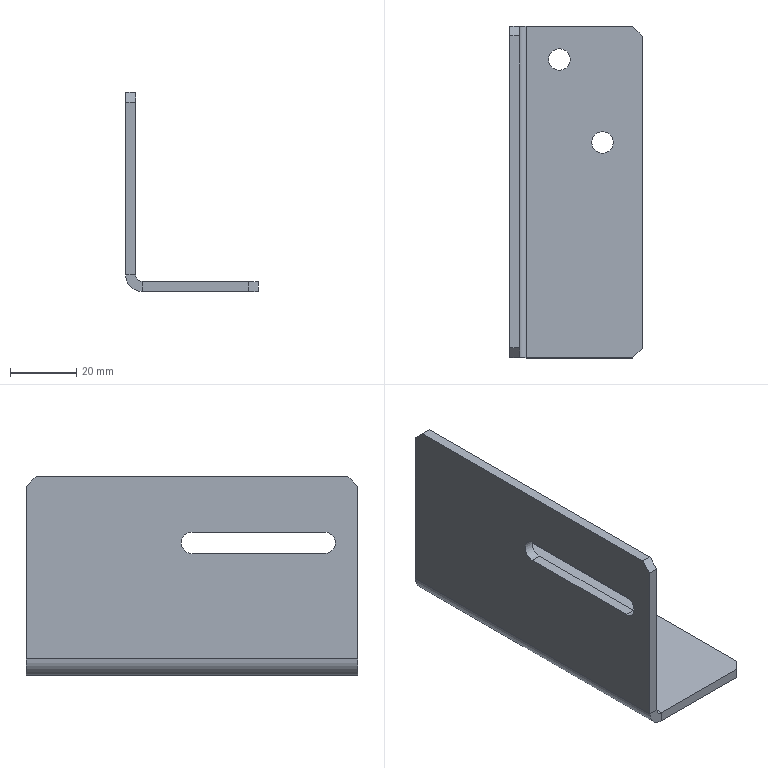Part | SolidWorks | features Chamfer 1, EdgeFlange 1, FlatPattern 1, ICE 1, SMBaseFlange 1, SheetMetal 1 | 1 solid | 26 faces | box 40 x 100 x 60 mm | volume 27517 mm3 | plane 18 | cylinder 8 | commonest cylinder face diameters 6.5 x6 4 x1 10 x1
STEP:
#1=CARTESIAN_POINT('',(-8.25,40.,-3.));
#2=VERTEX_POINT('',#1);
#3=CARTESIAN_POINT('',(-1.75,40.,-3.));
#4=VERTEX_POINT('',#3);
#5=CARTESIAN_POINT('',(-5.,40.,-3.));
#6=DIRECTION('',(0.,0.,1.));
#7=DIRECTION('',(1.,0.,0.));
#8=AXIS2_PLACEMENT_3D('',#5,#6,#7);
#9=CIRCLE('',#8,3.25);
#10=EDGE_CURVE('',#2,#4,#9,.T.);
#11=ORIENTED_EDGE('',*,*,#10,.F.);
#12=CARTESIAN_POINT('',(-8.25,40.,0.));
#13=VERTEX_POINT('',#12);
#14=CARTESIAN_POINT('',(-8.25,40.,-3.));
#15=DIRECTION('',(0.,0.,1.));
#16=VECTOR('',#15,1000.);
#17=LINE('',#14,#16);
#18=EDGE_CURVE('',#2,#13,#17,.T.);
#19=ORIENTED_EDGE('',*,*,#18,.T.);
#20=CARTESIAN_POINT('',(-1.75,40.,0.));
#21=VERTEX_POINT('',#20);
#22=CARTESIAN_POINT('',(-5.,40.,0.));
#23=DIRECTION('',(0.,0.,1.));
#24=DIRECTION('',(1.,0.,0.));
#25=AXIS2_PLACEMENT_3D('',#22,#23,#24);
#26=CIRCLE('',#25,3.25);
#27=EDGE_CURVE('',#13,#21,#26,.T.);
#28=ORIENTED_EDGE('',*,*,#27,.T.);
#29=CARTESIAN_POINT('',(-1.75,40.,-3.));
#30=DIRECTION('',(0.,0.,1.));
#31=VECTOR('',#30,1000.);
#32=LINE('',#29,#31);
#33=EDGE_CURVE('',#4,#21,#32,.T.);
#34=ORIENTED_EDGE('',*,*,#33,.F.);
#35=EDGE_LOOP('',(#11,#19,#28,#34));
#36=FACE_OUTER_BOUND('',#35,.T.);
#37=CARTESIAN_POINT('',(-5.,40.,-3.));
#38=DIRECTION('',(0.,0.,1.));
#39=DIRECTION('',(1.,0.,0.));
#40=AXIS2_PLACEMENT_3D('',#37,#38,#39);
#41=CYLINDRICAL_SURFACE('',#40,3.25);
#42=ADVANCED_FACE('',(#36),#41,.F.);
#43=CARTESIAN_POINT('',(4.75,15.,-3.));
#44=VERTEX_POINT('',#43);
#45=CARTESIAN_POINT('',(11.25,15.,-3.));
#46=VERTEX_POINT('',#45);
#47=CARTESIAN_POINT('',(8.,15.,-3.));
#48=DIRECTION('',(0.,0.,1.));
#49=DIRECTION('',(1.,0.,0.));
#50=AXIS2_PLACEMENT_3D('',#47,#48,#49);
#51=CIRCLE('',#50,3.25);
#52=EDGE_CURVE('',#44,#46,#51,.T.);
#53=ORIENTED_EDGE('',*,*,#52,.F.);
#54=CARTESIAN_POINT('',(4.75,15.,0.));
#55=VERTEX_POINT('',#54);
#56=CARTESIAN_POINT('',(4.75,15.,-3.));
#57=DIRECTION('',(0.,0.,1.));
#58=VECTOR('',#57,1000.);
#59=LINE('',#56,#58);
#60=EDGE_CURVE('',#44,#55,#59,.T.);
#61=ORIENTED_EDGE('',*,*,#60,.T.);
#62=CARTESIAN_POINT('',(11.25,15.,0.));
#63=VERTEX_POINT('',#62);
#64=CARTESIAN_POINT('',(8.,15.,0.));
#65=DIRECTION('',(0.,0.,1.));
#66=DIRECTION('',(1.,0.,0.));
#67=AXIS2_PLACEMENT_3D('',#64,#65,#66);
#68=CIRCLE('',#67,3.25);
#69=EDGE_CURVE('',#55,#63,#68,.T.);
#70=ORIENTED_EDGE('',*,*,#69,.T.);
#71=CARTESIAN_POINT('',(11.25,15.,-3.));
#72=DIRECTION('',(0.,0.,1.));
#73=VECTOR('',#72,1000.);
#74=LINE('',#71,#73);
#75=EDGE_CURVE('',#46,#63,#74,.T.);
#76=ORIENTED_EDGE('',*,*,#75,.F.);
#77=EDGE_LOOP('',(#53,#61,#70,#76));
#78=FACE_OUTER_BOUND('',#77,.T.);
#79=CARTESIAN_POINT('',(8.,15.,-3.));
#80=DIRECTION('',(0.,0.,1.));
#81=DIRECTION('',(1.,0.,0.));
#82=AXIS2_PLACEMENT_3D('',#79,#80,#81);
#83=CYLINDRICAL_SURFACE('',#82,3.25);
#84=ADVANCED_FACE('',(#78),#83,.F.);
#85=CARTESIAN_POINT('',(-15.,-50.,0.));
#86=VERTEX_POINT('',#85);
#87=CARTESIAN_POINT('',(17.,-50.,0.));
#88=VERTEX_POINT('',#87);
#89=CARTESIAN_POINT('',(17.,-50.,0.));
#90=DIRECTION('',(1.,0.,0.));
#91=VECTOR('',#90,1000.);
#92=LINE('',#89,#91);
#93=EDGE_CURVE('',#86,#88,#92,.T.);
#94=ORIENTED_EDGE('',*,*,#93,.F.);
#95=CARTESIAN_POINT('',(-15.,-50.,-3.));
#96=VERTEX_POINT('',#95);
#97=CARTESIAN_POINT('',(-15.,-50.,0.));
#98=DIRECTION('',(0.,0.,-1.));
#99=VECTOR('',#98,1000.);
#100=LINE('',#97,#99);
#101=EDGE_CURVE('',#86,#96,#100,.T.);
#102=ORIENTED_EDGE('',*,*,#101,.T.);
#103=CARTESIAN_POINT('',(17.,-50.,-3.));
#104=VERTEX_POINT('',#103);
#105=CARTESIAN_POINT('',(17.,-50.,-3.));
#106=DIRECTION('',(1.,0.,0.));
#107=VECTOR('',#106,1000.);
#108=LINE('',#105,#107);
#109=EDGE_CURVE('',#96,#104,#108,.T.);
#110=ORIENTED_EDGE('',*,*,#109,.T.);
#111=CARTESIAN_POINT('',(17.,-50.,-3.));
#112=DIRECTION('',(0.,0.,1.));
#113=VECTOR('',#112,1000.);
#114=LINE('',#111,#113);
#115=EDGE_CURVE('',#104,#88,#114,.T.);
#116=ORIENTED_EDGE('',*,*,#115,.T.);
#117=EDGE_LOOP('',(#94,#102,#110,#116));
#118=FACE_OUTER_BOUND('',#117,.T.);
#119=CARTESIAN_POINT('',(17.,-50.,-3.));
#120=DIRECTION('',(0.,-1.,0.));
#121=DIRECTION('',(0.,0.,-1.));
#122=AXIS2_PLACEMENT_3D('',#119,#120,#121);
#123=PLANE('',#122);
#124=ADVANCED_FACE('',(#118),#123,.T.);
#125=CARTESIAN_POINT('',(8.,15.,-3.));
#126=DIRECTION('',(0.,0.,1.));
#127=DIRECTION('',(1.,0.,0.));
#128=AXIS2_PLACEMENT_3D('',#125,#126,#127);
#129=CIRCLE('',#128,3.25);
#130=EDGE_CURVE('',#46,#44,#129,.T.);
#131=ORIENTED_EDGE('',*,*,#130,.T.);
#132=ORIENTED_EDGE('',*,*,#52,.T.);
#133=EDGE_LOOP('',(#131,#132));
#134=FACE_BOUND('',#133,.T.);
#135=CARTESIAN_POINT('',(-5.,40.,-3.));
#136=DIRECTION('',(0.,0.,1.));
#137=DIRECTION('',(1.,0.,0.));
#138=AXIS2_PLACEMENT_3D('',#135,#136,#137);
#139=CIRCLE('',#138,3.25);
#140=EDGE_CURVE('',#4,#2,#139,.T.);
#141=ORIENTED_EDGE('',*,*,#140,.T.);
#142=ORIENTED_EDGE('',*,*,#10,.T.);
#143=EDGE_LOOP('',(#141,#142));
#144=FACE_BOUND('',#143,.T.);
#145=CARTESIAN_POINT('',(-15.,50.,-3.));
#146=VERTEX_POINT('',#145);
#147=CARTESIAN_POINT('',(-15.,-50.,-3.));
#148=DIRECTION('',(0.,1.,0.));
#149=VECTOR('',#148,1000.);
#150=LINE('',#147,#149);
#151=EDGE_CURVE('',#96,#146,#150,.T.);
#152=ORIENTED_EDGE('',*,*,#151,.T.);
#153=CARTESIAN_POINT('',(17.,50.,-3.));
#154=VERTEX_POINT('',#153);
#155=CARTESIAN_POINT('',(17.,50.,-3.));
#156=DIRECTION('',(-1.,0.,0.));
#157=VECTOR('',#156,1000.);
#158=LINE('',#155,#157);
#159=EDGE_CURVE('',#154,#146,#158,.T.);
#160=ORIENTED_EDGE('',*,*,#159,.F.);
#161=CARTESIAN_POINT('',(20.,47.,-3.));
#162=VERTEX_POINT('',#161);
#163=CARTESIAN_POINT('',(20.,47.,-3.));
#164=DIRECTION('',(-0.7071,0.7071,0.));
#165=VECTOR('',#164,1000.);
#166=LINE('',#163,#165);
#167=EDGE_CURVE('',#162,#154,#166,.T.);
#168=ORIENTED_EDGE('',*,*,#167,.F.);
#169=CARTESIAN_POINT('',(20.,-47.,-3.));
#170=VERTEX_POINT('',#169);
#171=CARTESIAN_POINT('',(20.,-47.,-3.));
#172=DIRECTION('',(0.,1.,0.));
#173=VECTOR('',#172,1000.);
#174=LINE('',#171,#173);
#175=EDGE_CURVE('',#170,#162,#174,.T.);
#176=ORIENTED_EDGE('',*,*,#175,.F.);
#177=CARTESIAN_POINT('',(17.,-50.,-3.));
#178=DIRECTION('',(0.7071,0.7071,0.));
#179=VECTOR('',#178,1000.);
#180=LINE('',#177,#179);
#181=EDGE_CURVE('',#104,#170,#180,.T.);
#182=ORIENTED_EDGE('',*,*,#181,.F.);
#183=ORIENTED_EDGE('',*,*,#109,.F.);
#184=EDGE_LOOP('',(#152,#160,#168,#176,#182,#183));
#185=FACE_OUTER_BOUND('',#184,.T.);
#186=CARTESIAN_POINT('',(0.,0.,-3.));
#187=DIRECTION('',(0.,0.,1.));
#188=DIRECTION('',(1.,0.,0.));
#189=AXIS2_PLACEMENT_3D('',#186,#187,#188);
#190=PLANE('',#189);
#191=ADVANCED_FACE('',(#134,#144,#185),#190,.F.);
#192=CARTESIAN_POINT('',(-5.,40.,0.));
#193=DIRECTION('',(0.,0.,1.));
#194=DIRECTION('',(1.,0.,0.));
#195=AXIS2_PLACEMENT_3D('',#192,#193,#194);
#196=CIRCLE('',#195,3.25);
#197=EDGE_CURVE('',#21,#13,#196,.T.);
#198=ORIENTED_EDGE('',*,*,#197,.F.);
#199=ORIENTED_EDGE('',*,*,#27,.F.);
#200=EDGE_LOOP('',(#198,#199));
#201=FACE_BOUND('',#200,.T.);
#202=CARTESIAN_POINT('',(8.,15.,0.));
#203=DIRECTION('',(0.,0.,1.));
#204=DIRECTION('',(1.,0.,0.));
#205=AXIS2_PLACEMENT_3D('',#202,#203,#204);
#206=CIRCLE('',#205,3.25);
#207=EDGE_CURVE('',#63,#55,#206,.T.);
#208=ORIENTED_EDGE('',*,*,#207,.F.);
#209=ORIENTED_EDGE('',*,*,#69,.F.);
#210=EDGE_LOOP('',(#208,#209));
#211=FACE_BOUND('',#210,.T.);
#212=CARTESIAN_POINT('',(17.,50.,0.));
#213=VERTEX_POINT('',#212);
#214=CARTESIAN_POINT('',(-15.,50.,0.));
#215=VERTEX_POINT('',#214);
#216=CARTESIAN_POINT('',(17.,50.,0.));
#217=DIRECTION('',(-1.,0.,0.));
#218=VECTOR('',#217,1000.);
#219=LINE('',#216,#218);
#220=EDGE_CURVE('',#213,#215,#219,.T.);
#221=ORIENTED_EDGE('',*,*,#220,.T.);
#222=CARTESIAN_POINT('',(-15.,-50.,0.));
#223=DIRECTION('',(0.,1.,0.));
#224=VECTOR('',#223,1000.);
#225=LINE('',#222,#224);
#226=EDGE_CURVE('',#86,#215,#225,.T.);
#227=ORIENTED_EDGE('',*,*,#226,.F.);
#228=ORIENTED_EDGE('',*,*,#93,.T.);
#229=CARTESIAN_POINT('',(20.,-47.,0.));
#230=VERTEX_POINT('',#229);
#231=CARTESIAN_POINT('',(17.,-50.,0.));
#232=DIRECTION('',(0.7071,0.7071,0.));
#233=VECTOR('',#232,1000.);
#234=LINE('',#231,#233);
#235=EDGE_CURVE('',#88,#230,#234,.T.);
#236=ORIENTED_EDGE('',*,*,#235,.T.);
#237=CARTESIAN_POINT('',(20.,47.,0.));
#238=VERTEX_POINT('',#237);
#239=CARTESIAN_POINT('',(20.,-47.,0.));
#240=DIRECTION('',(0.,1.,0.));
#241=VECTOR('',#240,1000.);
#242=LINE('',#239,#241);
#243=EDGE_CURVE('',#230,#238,#242,.T.);
#244=ORIENTED_EDGE('',*,*,#243,.T.);
#245=CARTESIAN_POINT('',(20.,47.,0.));
#246=DIRECTION('',(-0.7071,0.7071,0.));
#247=VECTOR('',#246,1000.);
#248=LINE('',#245,#247);
#249=EDGE_CURVE('',#238,#213,#248,.T.);
#250=ORIENTED_EDGE('',*,*,#249,.T.);
#251=EDGE_LOOP('',(#221,#227,#228,#236,#244,#250));
#252=FACE_OUTER_BOUND('',#251,.T.);
#253=CARTESIAN_POINT('',(0.,0.,0.));
#254=DIRECTION('',(0.,0.,1.));
#255=DIRECTION('',(1.,0.,0.));
#256=AXIS2_PLACEMENT_3D('',#253,#254,#255);
#257=PLANE('',#256);
#258=ADVANCED_FACE('',(#201,#211,#252),#257,.T.);
#259=CARTESIAN_POINT('',(-15.,50.,0.));
#260=DIRECTION('',(0.,0.,-1.));
#261=VECTOR('',#260,1000.);
#262=LINE('',#259,#261);
#263=EDGE_CURVE('',#215,#146,#262,.T.);
#264=ORIENTED_EDGE('',*,*,#263,.F.);
#265=ORIENTED_EDGE('',*,*,#220,.F.);
#266=CARTESIAN_POINT('',(17.,50.,-3.));
#267=DIRECTION('',(0.,0.,1.));
#268=VECTOR('',#267,1000.);
#269=LINE('',#266,#268);
#270=EDGE_CURVE('',#154,#213,#269,.T.);
#271=ORIENTED_EDGE('',*,*,#270,.F.);
#272=ORIENTED_EDGE('',*,*,#159,.T.);
#273=EDGE_LOOP('',(#264,#265,#271,#272));
#274=FACE_OUTER_BOUND('',#273,.T.);
#275=CARTESIAN_POINT('',(17.,50.,-3.));
#276=DIRECTION('',(0.,1.,0.));
#277=DIRECTION('',(0.,0.,1.));
#278=AXIS2_PLACEMENT_3D('',#275,#276,#277);
#279=PLANE('',#278);
#280=ADVANCED_FACE('',(#274),#279,.T.);
#281=ORIENTED_EDGE('',*,*,#249,.F.);
#282=CARTESIAN_POINT('',(20.,47.,-3.));
#283=DIRECTION('',(0.,0.,1.));
#284=VECTOR('',#283,1000.);
#285=LINE('',#282,#284);
#286=EDGE_CURVE('',#162,#238,#285,.T.);
#287=ORIENTED_EDGE('',*,*,#286,.F.);
#288=ORIENTED_EDGE('',*,*,#167,.T.);
#289=ORIENTED_EDGE('',*,*,#270,.T.);
#290=EDGE_LOOP('',(#281,#287,#288,#289));
#291=FACE_OUTER_BOUND('',#290,.T.);
#292=CARTESIAN_POINT('',(20.,47.,-3.));
#293=DIRECTION('',(0.7071,0.7071,0.));
#294=DIRECTION('',(-0.7071,0.7071,0.));
#295=AXIS2_PLACEMENT_3D('',#292,#293,#294);
#296=PLANE('',#295);
#297=ADVANCED_FACE('',(#291),#296,.T.);
#298=ORIENTED_EDGE('',*,*,#243,.F.);
#299=CARTESIAN_POINT('',(20.,-47.,-3.));
#300=DIRECTION('',(0.,0.,1.));
#301=VECTOR('',#300,1000.);
#302=LINE('',#299,#301);
#303=EDGE_CURVE('',#170,#230,#302,.T.);
#304=ORIENTED_EDGE('',*,*,#303,.F.);
#305=ORIENTED_EDGE('',*,*,#175,.T.);
#306=ORIENTED_EDGE('',*,*,#286,.T.);
#307=EDGE_LOOP('',(#298,#304,#305,#306));
#308=FACE_OUTER_BOUND('',#307,.T.);
#309=CARTESIAN_POINT('',(20.,-47.,-3.));
#310=DIRECTION('',(1.,0.,0.));
#311=DIRECTION('',(0.,1.,0.));
#312=AXIS2_PLACEMENT_3D('',#309,#310,#311);
#313=PLANE('',#312);
#314=ADVANCED_FACE('',(#308),#313,.T.);
#315=ORIENTED_EDGE('',*,*,#235,.F.);
#316=ORIENTED_EDGE('',*,*,#115,.F.);
#317=ORIENTED_EDGE('',*,*,#181,.T.);
#318=ORIENTED_EDGE('',*,*,#303,.T.);
#319=EDGE_LOOP('',(#315,#316,#317,#318));
#320=FACE_OUTER_BOUND('',#319,.T.);
#321=CARTESIAN_POINT('',(17.,-50.,-3.));
#322=DIRECTION('',(0.7071,-0.7071,0.));
#323=DIRECTION('',(0.7071,0.7071,0.));
#324=AXIS2_PLACEMENT_3D('',#321,#322,#323);
#325=PLANE('',#324);
#326=ADVANCED_FACE('',(#320),#325,.T.);
#327=ORIENTED_EDGE('',*,*,#60,.F.);
#328=ORIENTED_EDGE('',*,*,#130,.F.);
#329=ORIENTED_EDGE('',*,*,#75,.T.);
#330=ORIENTED_EDGE('',*,*,#207,.T.);
#331=EDGE_LOOP('',(#327,#328,#329,#330));
#332=FACE_OUTER_BOUND('',#331,.T.);
#333=CARTESIAN_POINT('',(8.,15.,-3.));
#334=DIRECTION('',(0.,0.,1.));
#335=DIRECTION('',(1.,0.,0.));
#336=AXIS2_PLACEMENT_3D('',#333,#334,#335);
#337=CYLINDRICAL_SURFACE('',#336,3.25);
#338=ADVANCED_FACE('',(#332),#337,.F.);
#339=ORIENTED_EDGE('',*,*,#18,.F.);
#340=ORIENTED_EDGE('',*,*,#140,.F.);
#341=ORIENTED_EDGE('',*,*,#33,.T.);
#342=ORIENTED_EDGE('',*,*,#197,.T.);
#343=EDGE_LOOP('',(#339,#340,#341,#342));
#344=FACE_OUTER_BOUND('',#343,.T.);
#345=CARTESIAN_POINT('',(-5.,40.,-3.));
#346=DIRECTION('',(0.,0.,1.));
#347=DIRECTION('',(1.,0.,0.));
#348=AXIS2_PLACEMENT_3D('',#345,#346,#347);
#349=CYLINDRICAL_SURFACE('',#348,3.25);
#350=ADVANCED_FACE('',(#344),#349,.F.);
#351=CARTESIAN_POINT('',(-17.,50.,2.));
#352=VERTEX_POINT('',#351);
#353=CARTESIAN_POINT('',(-20.,50.,2.));
#354=VERTEX_POINT('',#353);
#355=CARTESIAN_POINT('',(-20.,50.,2.));
#356=DIRECTION('',(-1.,0.,0.));
#357=VECTOR('',#356,1000.);
#358=LINE('',#355,#357);
#359=EDGE_CURVE('',#352,#354,#358,.T.);
#360=ORIENTED_EDGE('',*,*,#359,.F.);
#361=CARTESIAN_POINT('',(-15.,50.,2.));
#362=DIRECTION('',(0.,1.,0.));
#363=DIRECTION('',(0.,0.,-1.));
#364=AXIS2_PLACEMENT_3D('',#361,#362,#363);
#365=CIRCLE('',#364,2.);
#366=EDGE_CURVE('',#215,#352,#365,.T.);
#367=ORIENTED_EDGE('',*,*,#366,.F.);
#368=ORIENTED_EDGE('',*,*,#263,.T.);
#369=CARTESIAN_POINT('',(-15.,50.,2.));
#370=DIRECTION('',(0.,1.,0.));
#371=DIRECTION('',(0.,0.,-1.));
#372=AXIS2_PLACEMENT_3D('',#369,#370,#371);
#373=CIRCLE('',#372,5.);
#374=EDGE_CURVE('',#146,#354,#373,.T.);
#375=ORIENTED_EDGE('',*,*,#374,.T.);
#376=EDGE_LOOP('',(#360,#367,#368,#375));
#377=FACE_OUTER_BOUND('',#376,.T.);
#378=CARTESIAN_POINT('',(-15.,50.,2.));
#379=DIRECTION('',(0.,1.,0.));
#380=DIRECTION('',(0.,0.,1.));
#381=AXIS2_PLACEMENT_3D('',#378,#379,#380);
#382=PLANE('',#381);
#383=ADVANCED_FACE('',(#377),#382,.T.);
#384=CARTESIAN_POINT('',(-17.,-50.,2.));
#385=VERTEX_POINT('',#384);
#386=CARTESIAN_POINT('',(-15.,-50.,2.));
#387=DIRECTION('',(0.,-1.,0.));
#388=DIRECTION('',(0.,0.,-1.));
#389=AXIS2_PLACEMENT_3D('',#386,#387,#388);
#390=CIRCLE('',#389,2.);
#391=EDGE_CURVE('',#385,#86,#390,.T.);
#392=ORIENTED_EDGE('',*,*,#391,.F.);
#393=CARTESIAN_POINT('',(-20.,-50.,2.));
#394=VERTEX_POINT('',#393);
#395=CARTESIAN_POINT('',(-17.,-50.,2.));
#396=DIRECTION('',(-1.,0.,0.));
#397=VECTOR('',#396,1000.);
#398=LINE('',#395,#397);
#399=EDGE_CURVE('',#385,#394,#398,.T.);
#400=ORIENTED_EDGE('',*,*,#399,.T.);
#401=CARTESIAN_POINT('',(-15.,-50.,2.));
#402=DIRECTION('',(0.,-1.,0.));
#403=DIRECTION('',(0.,0.,-1.));
#404=AXIS2_PLACEMENT_3D('',#401,#402,#403);
#405=CIRCLE('',#404,5.);
#406=EDGE_CURVE('',#394,#96,#405,.T.);
#407=ORIENTED_EDGE('',*,*,#406,.T.);
#408=ORIENTED_EDGE('',*,*,#101,.F.);
#409=EDGE_LOOP('',(#392,#400,#407,#408));
#410=FACE_OUTER_BOUND('',#409,.T.);
#411=CARTESIAN_POINT('',(-15.,-50.,2.));
#412=DIRECTION('',(0.,1.,0.));
#413=DIRECTION('',(0.,0.,1.));
#414=AXIS2_PLACEMENT_3D('',#411,#412,#413);
#415=PLANE('',#414);
#416=ADVANCED_FACE('',(#410),#415,.F.);
#417=ORIENTED_EDGE('',*,*,#151,.F.);
#418=ORIENTED_EDGE('',*,*,#406,.F.);
#419=CARTESIAN_POINT('',(-20.,0.,2.));
#420=DIRECTION('',(0.,-1.,0.));
#421=VECTOR('',#420,1000.);
#422=LINE('',#419,#421);
#423=EDGE_CURVE('',#354,#394,#422,.T.);
#424=ORIENTED_EDGE('',*,*,#423,.F.);
#425=ORIENTED_EDGE('',*,*,#374,.F.);
#426=EDGE_LOOP('',(#417,#418,#424,#425));
#427=FACE_OUTER_BOUND('',#426,.T.);
#428=CARTESIAN_POINT('',(-15.,-50.,2.));
#429=DIRECTION('',(0.,-1.,0.));
#430=DIRECTION('',(-1.,0.,0.));
#431=AXIS2_PLACEMENT_3D('',#428,#429,#430);
#432=CYLINDRICAL_SURFACE('',#431,5.);
#433=ADVANCED_FACE('',(#427),#432,.T.);
#434=ORIENTED_EDGE('',*,*,#226,.T.);
#435=ORIENTED_EDGE('',*,*,#366,.T.);
#436=CARTESIAN_POINT('',(-17.,50.,2.));
#437=DIRECTION('',(0.,-1.,0.));
#438=VECTOR('',#437,1000.);
#439=LINE('',#436,#438);
#440=EDGE_CURVE('',#352,#385,#439,.T.);
#441=ORIENTED_EDGE('',*,*,#440,.T.);
#442=ORIENTED_EDGE('',*,*,#391,.T.);
#443=EDGE_LOOP('',(#434,#435,#441,#442));
#444=FACE_OUTER_BOUND('',#443,.T.);
#445=CARTESIAN_POINT('',(-15.,-50.,2.));
#446=DIRECTION('',(0.,-1.,0.));
#447=DIRECTION('',(-1.,0.,0.));
#448=AXIS2_PLACEMENT_3D('',#445,#446,#447);
#449=CYLINDRICAL_SURFACE('',#448,2.);
#450=ADVANCED_FACE('',(#444),#449,.F.);
#451=CARTESIAN_POINT('',(-17.,-50.,54.));
#452=VERTEX_POINT('',#451);
#453=CARTESIAN_POINT('',(-17.,-50.,0.));
#454=DIRECTION('',(0.,0.,-1.));
#455=VECTOR('',#454,1000.);
#456=LINE('',#453,#455);
#457=EDGE_CURVE('',#452,#385,#456,.T.);
#458=ORIENTED_EDGE('',*,*,#457,.F.);
#459=CARTESIAN_POINT('',(-20.,-50.,54.));
#460=VERTEX_POINT('',#459);
#461=CARTESIAN_POINT('',(-20.,-50.,54.));
#462=DIRECTION('',(-1.,0.,0.));
#463=VECTOR('',#462,1000.);
#464=LINE('',#461,#463);
#465=EDGE_CURVE('',#452,#460,#464,.T.);
#466=ORIENTED_EDGE('',*,*,#465,.T.);
#467=CARTESIAN_POINT('',(-20.,-50.,0.));
#468=DIRECTION('',(0.,0.,-1.));
#469=VECTOR('',#468,1000.);
#470=LINE('',#467,#469);
#471=EDGE_CURVE('',#460,#394,#470,.T.);
#472=ORIENTED_EDGE('',*,*,#471,.T.);
#473=ORIENTED_EDGE('',*,*,#399,.F.);
#474=EDGE_LOOP('',(#458,#466,#472,#473));
#475=FACE_OUTER_BOUND('',#474,.T.);
#476=CARTESIAN_POINT('',(-20.,-50.,0.));
#477=DIRECTION('',(0.,-1.,0.));
#478=DIRECTION('',(0.,0.,-1.));
#479=AXIS2_PLACEMENT_3D('',#476,#477,#478);
#480=PLANE('',#479);
#481=ADVANCED_FACE('',(#475),#480,.T.);
#482=CARTESIAN_POINT('',(-20.,50.,54.));
#483=VERTEX_POINT('',#482);
#484=CARTESIAN_POINT('',(-20.,50.,57.));
#485=DIRECTION('',(0.,0.,1.));
#486=VECTOR('',#485,1000.);
#487=LINE('',#484,#486);
#488=EDGE_CURVE('',#354,#483,#487,.T.);
#489=ORIENTED_EDGE('',*,*,#488,.T.);
#490=CARTESIAN_POINT('',(-17.,50.,54.));
#491=VERTEX_POINT('',#490);
#492=CARTESIAN_POINT('',(-20.,50.,54.));
#493=DIRECTION('',(1.,0.,0.));
#494=VECTOR('',#493,1000.);
#495=LINE('',#492,#494);
#496=EDGE_CURVE('',#483,#491,#495,.T.);
#497=ORIENTED_EDGE('',*,*,#496,.T.);
#498=CARTESIAN_POINT('',(-17.,50.,0.));
#499=DIRECTION('',(0.,0.,1.));
#500=VECTOR('',#499,1000.);
#501=LINE('',#498,#500);
#502=EDGE_CURVE('',#352,#491,#501,.T.);
#503=ORIENTED_EDGE('',*,*,#502,.F.);
#504=ORIENTED_EDGE('',*,*,#359,.T.);
#505=EDGE_LOOP('',(#489,#497,#503,#504));
#506=FACE_OUTER_BOUND('',#505,.T.);
#507=CARTESIAN_POINT('',(-20.,50.,57.));
#508=DIRECTION('',(0.,1.,0.));
#509=DIRECTION('',(0.,0.,1.));
#510=AXIS2_PLACEMENT_3D('',#507,#508,#509);
#511=PLANE('',#510);
#512=ADVANCED_FACE('',(#506),#511,.T.);
#513=CARTESIAN_POINT('',(-20.,-40.,33.75));
#514=VERTEX_POINT('',#513);
#515=CARTESIAN_POINT('',(-20.,-40.,40.25));
#516=VERTEX_POINT('',#515);
#517=CARTESIAN_POINT('',(-20.,-40.,37.));
#518=DIRECTION('',(-1.,0.,0.));
#519=DIRECTION('',(0.,0.,1.));
#520=AXIS2_PLACEMENT_3D('',#517,#518,#519);
#521=CIRCLE('',#520,3.25);
#522=EDGE_CURVE('',#514,#516,#521,.T.);
#523=ORIENTED_EDGE('',*,*,#522,.F.);
#524=CARTESIAN_POINT('',(-20.,0.,33.75));
#525=VERTEX_POINT('',#524);
#526=CARTESIAN_POINT('',(-20.,-40.,33.75));
#527=DIRECTION('',(0.,-1.,0.));
#528=VECTOR('',#527,1000.);
#529=LINE('',#526,#528);
#530=EDGE_CURVE('',#525,#514,#529,.T.);
#531=ORIENTED_EDGE('',*,*,#530,.F.);
#532=CARTESIAN_POINT('',(-20.,0.,40.25));
#533=VERTEX_POINT('',#532);
#534=CARTESIAN_POINT('',(-20.,0.,37.));
#535=DIRECTION('',(-1.,0.,0.));
#536=DIRECTION('',(0.,0.,1.));
#537=AXIS2_PLACEMENT_3D('',#534,#535,#536);
#538=CIRCLE('',#537,3.25);
#539=EDGE_CURVE('',#533,#525,#538,.T.);
#540=ORIENTED_EDGE('',*,*,#539,.F.);
#541=CARTESIAN_POINT('',(-20.,-40.,40.25));
#542=DIRECTION('',(0.,1.,0.));
#543=VECTOR('',#542,1000.);
#544=LINE('',#541,#543);
#545=EDGE_CURVE('',#516,#533,#544,.T.);
#546=ORIENTED_EDGE('',*,*,#545,.F.);
#547=EDGE_LOOP('',(#523,#531,#540,#546));
#548=FACE_BOUND('',#547,.T.);
#549=CARTESIAN_POINT('',(-20.,47.,57.));
#550=VERTEX_POINT('',#549);
#551=CARTESIAN_POINT('',(-20.,-47.,57.));
#552=VERTEX_POINT('',#551);
#553=CARTESIAN_POINT('',(-20.,-50.,57.));
#554=DIRECTION('',(0.,-1.,0.));
#555=VECTOR('',#554,1000.);
#556=LINE('',#553,#555);
#557=EDGE_CURVE('',#550,#552,#556,.T.);
#558=ORIENTED_EDGE('',*,*,#557,.F.);
#559=CARTESIAN_POINT('',(-20.,52.,52.));
#560=DIRECTION('',(0.,0.7071,-0.7071));
#561=VECTOR('',#560,1000.);
#562=LINE('',#559,#561);
#563=EDGE_CURVE('',#550,#483,#562,.T.);
#564=ORIENTED_EDGE('',*,*,#563,.T.);
#565=ORIENTED_EDGE('',*,*,#488,.F.);
#566=ORIENTED_EDGE('',*,*,#423,.T.);
#567=ORIENTED_EDGE('',*,*,#471,.F.);
#568=CARTESIAN_POINT('',(-20.,-52.,52.));
#569=DIRECTION('',(0.,0.7071,0.7071));
#570=VECTOR('',#569,1000.);
#571=LINE('',#568,#570);
#572=EDGE_CURVE('',#460,#552,#571,.T.);
#573=ORIENTED_EDGE('',*,*,#572,.T.);
#574=EDGE_LOOP('',(#558,#564,#565,#566,#567,#573));
#575=FACE_OUTER_BOUND('',#574,.T.);
#576=CARTESIAN_POINT('',(-20.,0.,0.));
#577=DIRECTION('',(-1.,0.,0.));
#578=DIRECTION('',(0.,0.,1.));
#579=AXIS2_PLACEMENT_3D('',#576,#577,#578);
#580=PLANE('',#579);
#581=ADVANCED_FACE('',(#548,#575),#580,.T.);
#582=CARTESIAN_POINT('',(-17.,0.,33.75));
#583=VERTEX_POINT('',#582);
#584=CARTESIAN_POINT('',(-17.,-40.,33.75));
#585=VERTEX_POINT('',#584);
#586=CARTESIAN_POINT('',(-17.,0.,33.75));
#587=DIRECTION('',(0.,-1.,0.));
#588=VECTOR('',#587,1000.);
#589=LINE('',#586,#588);
#590=EDGE_CURVE('',#583,#585,#589,.T.);
#591=ORIENTED_EDGE('',*,*,#590,.T.);
#592=CARTESIAN_POINT('',(-17.,-40.,40.25));
#593=VERTEX_POINT('',#592);
#594=CARTESIAN_POINT('',(-17.,-40.,37.));
#595=DIRECTION('',(-1.,0.,0.));
#596=DIRECTION('',(0.,0.,1.));
#597=AXIS2_PLACEMENT_3D('',#594,#595,#596);
#598=CIRCLE('',#597,3.25);
#599=EDGE_CURVE('',#585,#593,#598,.T.);
#600=ORIENTED_EDGE('',*,*,#599,.T.);
#601=CARTESIAN_POINT('',(-17.,0.,40.25));
#602=VERTEX_POINT('',#601);
#603=CARTESIAN_POINT('',(-17.,0.,40.25));
#604=DIRECTION('',(0.,1.,0.));
#605=VECTOR('',#604,1000.);
#606=LINE('',#603,#605);
#607=EDGE_CURVE('',#593,#602,#606,.T.);
#608=ORIENTED_EDGE('',*,*,#607,.T.);
#609=CARTESIAN_POINT('',(-17.,0.,37.));
#610=DIRECTION('',(-1.,0.,0.));
#611=DIRECTION('',(0.,0.,1.));
#612=AXIS2_PLACEMENT_3D('',#609,#610,#611);
#613=CIRCLE('',#612,3.25);
#614=EDGE_CURVE('',#602,#583,#613,.T.);
#615=ORIENTED_EDGE('',*,*,#614,.T.);
#616=EDGE_LOOP('',(#591,#600,#608,#615));
#617=FACE_BOUND('',#616,.T.);
#618=ORIENTED_EDGE('',*,*,#502,.T.);
#619=CARTESIAN_POINT('',(-17.,47.,57.));
#620=VERTEX_POINT('',#619);
#621=CARTESIAN_POINT('',(-17.,50.,54.));
#622=DIRECTION('',(0.,-0.7071,0.7071));
#623=VECTOR('',#622,1000.);
#624=LINE('',#621,#623);
#625=EDGE_CURVE('',#491,#620,#624,.T.);
#626=ORIENTED_EDGE('',*,*,#625,.T.);
#627=CARTESIAN_POINT('',(-17.,-47.,57.));
#628=VERTEX_POINT('',#627);
#629=CARTESIAN_POINT('',(-17.,0.,57.));
#630=DIRECTION('',(0.,-1.,0.));
#631=VECTOR('',#630,1000.);
#632=LINE('',#629,#631);
#633=EDGE_CURVE('',#620,#628,#632,.T.);
#634=ORIENTED_EDGE('',*,*,#633,.T.);
#635=CARTESIAN_POINT('',(-17.,-47.,57.));
#636=DIRECTION('',(0.,-0.7071,-0.7071));
#637=VECTOR('',#636,1000.);
#638=LINE('',#635,#637);
#639=EDGE_CURVE('',#628,#452,#638,.T.);
#640=ORIENTED_EDGE('',*,*,#639,.T.);
#641=ORIENTED_EDGE('',*,*,#457,.T.);
#642=ORIENTED_EDGE('',*,*,#440,.F.);
#643=EDGE_LOOP('',(#618,#626,#634,#640,#641,#642));
#644=FACE_OUTER_BOUND('',#643,.T.);
#645=CARTESIAN_POINT('',(-17.,0.,0.));
#646=DIRECTION('',(-1.,0.,0.));
#647=DIRECTION('',(0.,0.,1.));
#648=AXIS2_PLACEMENT_3D('',#645,#646,#647);
#649=PLANE('',#648);
#650=ADVANCED_FACE('',(#617,#644),#649,.F.);
#651=ORIENTED_EDGE('',*,*,#633,.F.);
#652=CARTESIAN_POINT('',(-20.,47.,57.));
#653=DIRECTION('',(-1.,0.,0.));
#654=VECTOR('',#653,1000.);
#655=LINE('',#652,#654);
#656=EDGE_CURVE('',#620,#550,#655,.T.);
#657=ORIENTED_EDGE('',*,*,#656,.T.);
#658=ORIENTED_EDGE('',*,*,#557,.T.);
#659=CARTESIAN_POINT('',(-20.,-47.,57.));
#660=DIRECTION('',(1.,0.,0.));
#661=VECTOR('',#660,1000.);
#662=LINE('',#659,#661);
#663=EDGE_CURVE('',#552,#628,#662,.T.);
#664=ORIENTED_EDGE('',*,*,#663,.T.);
#665=EDGE_LOOP('',(#651,#657,#658,#664));
#666=FACE_OUTER_BOUND('',#665,.T.);
#667=CARTESIAN_POINT('',(-20.,-50.,57.));
#668=DIRECTION('',(0.,0.,1.));
#669=DIRECTION('',(1.,0.,0.));
#670=AXIS2_PLACEMENT_3D('',#667,#668,#669);
#671=PLANE('',#670);
#672=ADVANCED_FACE('',(#666),#671,.T.);
#673=ORIENTED_EDGE('',*,*,#563,.F.);
#674=ORIENTED_EDGE('',*,*,#656,.F.);
#675=ORIENTED_EDGE('',*,*,#625,.F.);
#676=ORIENTED_EDGE('',*,*,#496,.F.);
#677=EDGE_LOOP('',(#673,#674,#675,#676));
#678=FACE_OUTER_BOUND('',#677,.T.);
#679=CARTESIAN_POINT('',(-20.,50.,54.));
#680=DIRECTION('',(0.,-0.7071,-0.7071));
#681=DIRECTION('',(1.,0.,0.));
#682=AXIS2_PLACEMENT_3D('',#679,#680,#681);
#683=PLANE('',#682);
#684=ADVANCED_FACE('',(#678),#683,.F.);
#685=ORIENTED_EDGE('',*,*,#572,.F.);
#686=ORIENTED_EDGE('',*,*,#465,.F.);
#687=ORIENTED_EDGE('',*,*,#639,.F.);
#688=ORIENTED_EDGE('',*,*,#663,.F.);
#689=EDGE_LOOP('',(#685,#686,#687,#688));
#690=FACE_OUTER_BOUND('',#689,.T.);
#691=CARTESIAN_POINT('',(-20.,-47.,57.));
#692=DIRECTION('',(0.,0.7071,-0.7071));
#693=DIRECTION('',(1.,0.,0.));
#694=AXIS2_PLACEMENT_3D('',#691,#692,#693);
#695=PLANE('',#694);
#696=ADVANCED_FACE('',(#690),#695,.F.);
#697=CARTESIAN_POINT('',(20.,-40.,33.75));
#698=DIRECTION('',(-1.,0.,0.));
#699=VECTOR('',#698,1000.);
#700=LINE('',#697,#699);
#701=EDGE_CURVE('',#585,#514,#700,.T.);
#702=ORIENTED_EDGE('',*,*,#701,.T.);
#703=ORIENTED_EDGE('',*,*,#522,.T.);
#704=CARTESIAN_POINT('',(20.,-40.,40.25));
#705=DIRECTION('',(-1.,0.,0.));
#706=VECTOR('',#705,1000.);
#707=LINE('',#704,#706);
#708=EDGE_CURVE('',#593,#516,#707,.T.);
#709=ORIENTED_EDGE('',*,*,#708,.F.);
#710=ORIENTED_EDGE('',*,*,#599,.F.);
#711=EDGE_LOOP('',(#702,#703,#709,#710));
#712=FACE_OUTER_BOUND('',#711,.T.);
#713=CARTESIAN_POINT('',(20.,-40.,37.));
#714=DIRECTION('',(-1.,0.,0.));
#715=DIRECTION('',(0.,0.,1.));
#716=AXIS2_PLACEMENT_3D('',#713,#714,#715);
#717=CYLINDRICAL_SURFACE('',#716,3.25);
#718=ADVANCED_FACE('',(#712),#717,.F.);
#719=CARTESIAN_POINT('',(20.,0.,33.75));
#720=DIRECTION('',(-1.,0.,0.));
#721=VECTOR('',#720,1000.);
#722=LINE('',#719,#721);
#723=EDGE_CURVE('',#583,#525,#722,.T.);
#724=ORIENTED_EDGE('',*,*,#723,.T.);
#725=ORIENTED_EDGE('',*,*,#530,.T.);
#726=ORIENTED_EDGE('',*,*,#701,.F.);
#727=ORIENTED_EDGE('',*,*,#590,.F.);
#728=EDGE_LOOP('',(#724,#725,#726,#727));
#729=FACE_OUTER_BOUND('',#728,.T.);
#730=CARTESIAN_POINT('',(20.,-40.,33.75));
#731=DIRECTION('',(0.,0.,-1.));
#732=DIRECTION('',(-1.,0.,0.));
#733=AXIS2_PLACEMENT_3D('',#730,#731,#732);
#734=PLANE('',#733);
#735=ADVANCED_FACE('',(#729),#734,.F.);
#736=CARTESIAN_POINT('',(20.,0.,40.25));
#737=DIRECTION('',(-1.,0.,0.));
#738=VECTOR('',#737,1000.);
#739=LINE('',#736,#738);
#740=EDGE_CURVE('',#602,#533,#739,.T.);
#741=ORIENTED_EDGE('',*,*,#740,.T.);
#742=ORIENTED_EDGE('',*,*,#539,.T.);
#743=ORIENTED_EDGE('',*,*,#723,.F.);
#744=ORIENTED_EDGE('',*,*,#614,.F.);
#745=EDGE_LOOP('',(#741,#742,#743,#744));
#746=FACE_OUTER_BOUND('',#745,.T.);
#747=CARTESIAN_POINT('',(20.,0.,37.));
#748=DIRECTION('',(-1.,0.,0.));
#749=DIRECTION('',(0.,0.,1.));
#750=AXIS2_PLACEMENT_3D('',#747,#748,#749);
#751=CYLINDRICAL_SURFACE('',#750,3.25);
#752=ADVANCED_FACE('',(#746),#751,.F.);
#753=ORIENTED_EDGE('',*,*,#708,.T.);
#754=ORIENTED_EDGE('',*,*,#545,.T.);
#755=ORIENTED_EDGE('',*,*,#740,.F.);
#756=ORIENTED_EDGE('',*,*,#607,.F.);
#757=EDGE_LOOP('',(#753,#754,#755,#756));
#758=FACE_OUTER_BOUND('',#757,.T.);
#759=CARTESIAN_POINT('',(20.,-40.,40.25));
#760=DIRECTION('',(0.,0.,1.));
#761=DIRECTION('',(1.,0.,0.));
#762=AXIS2_PLACEMENT_3D('',#759,#760,#761);
#763=PLANE('',#762);
#764=ADVANCED_FACE('',(#758),#763,.F.);
#765=CLOSED_SHELL('',(#42,#84,#124,#191,#258,#280,#297,#314,#326,#338,#350,#383,#416,#433,#450,#481,#512,#581,#650,#672,#684,#696,#718,#735,#752,#764));
#766=MANIFOLD_SOLID_BREP('',#765);
#767=CARTESIAN_POINT('',(0.,0.,0.));
#768=DIRECTION('',(0.,0.,1.));
#769=DIRECTION('',(1.,0.,0.));
#770=AXIS2_PLACEMENT_3D('',#767,#768,#769);
#771=(LENGTH_UNIT()NAMED_UNIT(*)SI_UNIT(.MILLI.,.METRE.));
#772=UNCERTAINTY_MEASURE_WITH_UNIT(LENGTH_MEASURE(0.00001),#771,'','');
#773=(NAMED_UNIT(*)PLANE_ANGLE_UNIT()SI_UNIT($,.RADIAN.));
#774=(NAMED_UNIT(*)SI_UNIT($,.STERADIAN.)SOLID_ANGLE_UNIT());
#775=(GEOMETRIC_REPRESENTATION_CONTEXT(3)GLOBAL_UNCERTAINTY_ASSIGNED_CONTEXT((#772))GLOBAL_UNIT_ASSIGNED_CONTEXT((#771,#773,#774))REPRESENTATION_CONTEXT('',''));
#776=ADVANCED_BREP_SHAPE_REPRESENTATION('',(#766,#770),#775);